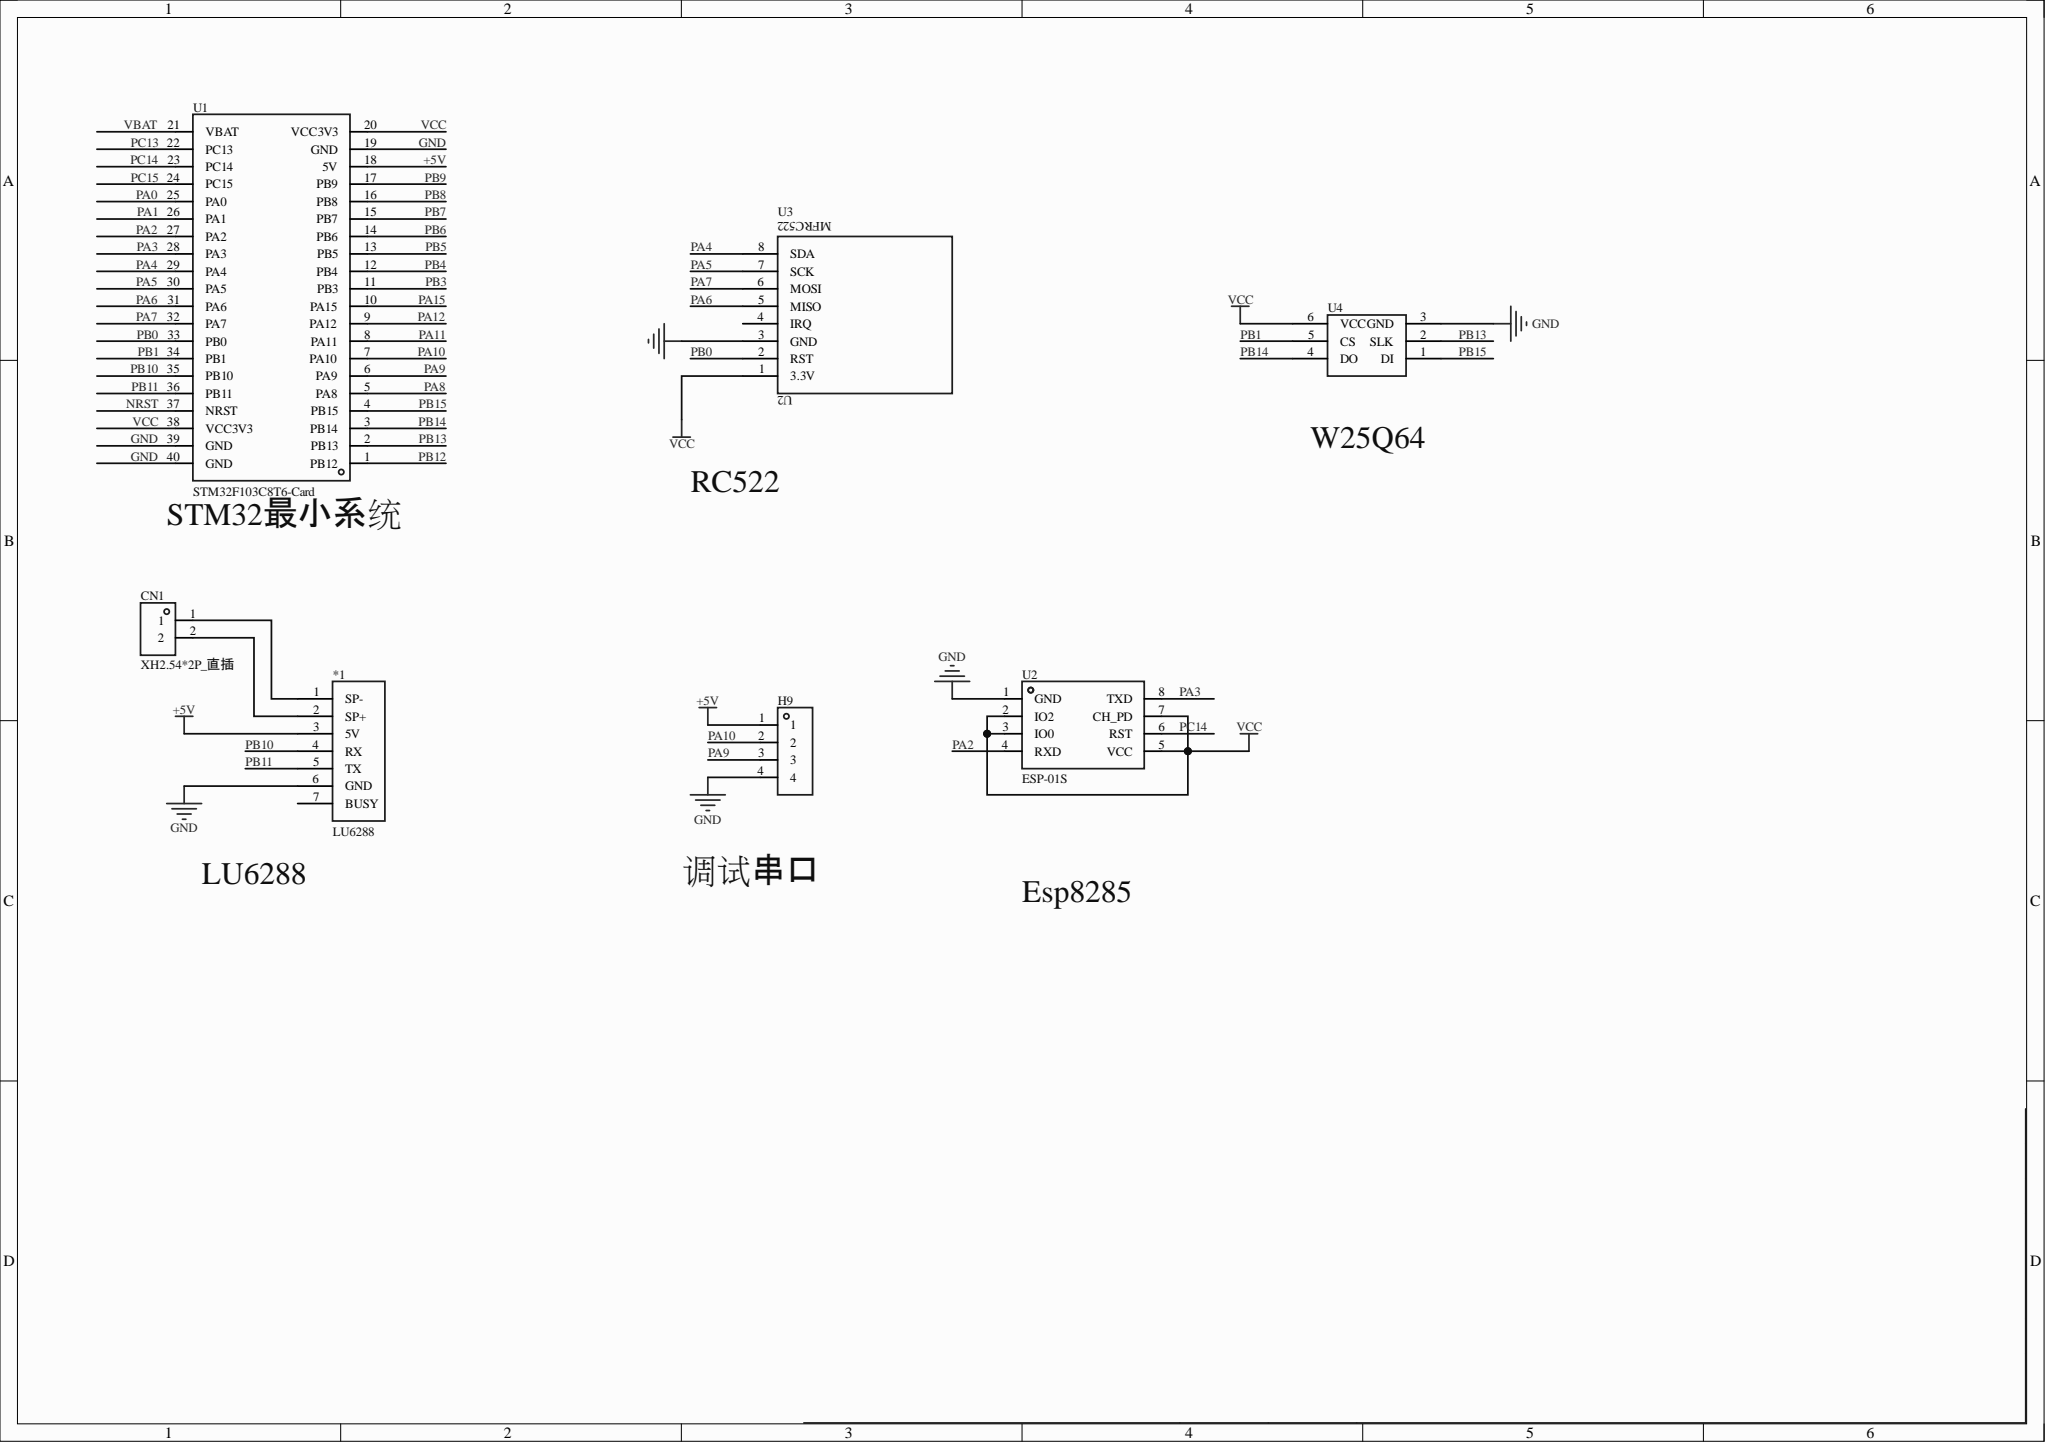Circuit board | Altium Designer | 7 parts | 21 nets
Bill of materials:
Comment,Description,Designator,Footprint,LibRef,Quantity
"LU6288","","*1","LU6288","LU6288","1"
"XH2.54*2P_直插","","CN1","CONN-TH_2P-P2.50-XH2.54-2P","XH2.54*2P_直插","1"
"","","H9","HDR-TH_4P-P2.54-V-M","HDR-M_2.54_1x4P","1"
"STM32F103C8T6-Card","","U1","CONN-TH_L53.3-W22.9_STM32F103C8T6-CARD","STM32F103C8T6-Card","1"
"ESP-01S","","U2","WIFIM-TH_ESP-01S","ESP-01S_C111009","1"
"","","U3","RC522","RC522","1"
"","","U4","W25Q64","W25Q64","1"
Netlist (Protel format):
[
*1
LU6288
LU6288



]
[
CN1
CONN-TH_2P-P2.50-XH2.54-2P
XH2.54*2P_直插



]
[
H9
HDR-TH_4P-P2.54-V-M




]
[
U1
CONN-TH_L53.3-W22.9_STM32F103C8T6-CARD
STM32F103C8T6-Card



]
[
U2
WIFIM-TH_ESP-01S
ESP-01S



]
[
U3
RC522




]
[
U4
W25Q64




]
(
VCC
U1-20
U1-38
U2-2
U2-3
U2-5
U2-7
U3-1
U4-6
)
(
PC14
U1-23
U2-6
)
(
PB15
U1-4
U4-1
)
(
PB14
U1-3
U4-4
)
(
PB13
U1-2
U4-2
)
(
PB11
*1-5
U1-36
)
(
PB10
*1-4
U1-35
)
(
PB1
U1-34
U4-5
)
(
PB0
U1-33
U3-2
)
(
PA10
H9-2
U1-7
)
(
PA9
H9-3
U1-6
)
(
PA7
U1-32
U3-6
)
(
PA6
U1-31
U3-5
)
(
PA5
U1-30
U3-7
)
(
PA4
U1-29
U3-8
)
(
PA3
U1-28
U2-8
)
(
PA2
U1-27
U2-4
)
(
Net*1_2
*1-2
CN1-2
)
(
Net*1_1
*1-1
CN1-1
)
(
GND
*1-6
H9-4
U1-19
U1-39
U1-40
U2-1
U3-3
U4-3
)
(
+5V
*1-3
H9-1
U1-18
)